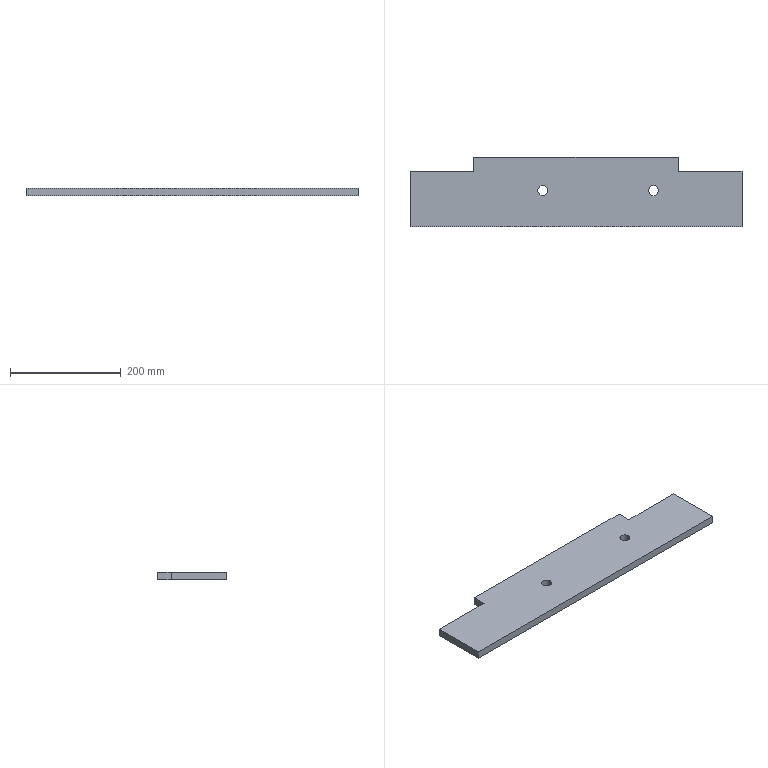Part | SolidWorks | features Extrusion 1 | 1 solid | 14 faces | box 600 x 125 x 14 mm | volume 962375 mm3 | plane 10 | cylinder 4 | commonest cylinder face diameters 18 x4
STEP:
#1=CARTESIAN_POINT('',(431.,65.,14.));
#2=VERTEX_POINT('',#1);
#3=CARTESIAN_POINT('',(449.,65.,14.));
#4=VERTEX_POINT('',#3);
#5=CARTESIAN_POINT('',(440.,65.,14.));
#6=DIRECTION('',(0.,0.,1.));
#7=DIRECTION('',(1.,0.,0.));
#8=AXIS2_PLACEMENT_3D('',#5,#6,#7);
#9=CIRCLE('',#8,9.);
#10=EDGE_CURVE('',#2,#4,#9,.T.);
#11=ORIENTED_EDGE('',*,*,#10,.T.);
#12=CARTESIAN_POINT('',(449.,65.,0.));
#13=VERTEX_POINT('',#12);
#14=CARTESIAN_POINT('',(449.,65.,14.));
#15=DIRECTION('',(0.,0.,-1.));
#16=VECTOR('',#15,1000.);
#17=LINE('',#14,#16);
#18=EDGE_CURVE('',#4,#13,#17,.T.);
#19=ORIENTED_EDGE('',*,*,#18,.T.);
#20=CARTESIAN_POINT('',(431.,65.,0.));
#21=VERTEX_POINT('',#20);
#22=CARTESIAN_POINT('',(440.,65.,0.));
#23=DIRECTION('',(0.,0.,1.));
#24=DIRECTION('',(1.,0.,0.));
#25=AXIS2_PLACEMENT_3D('',#22,#23,#24);
#26=CIRCLE('',#25,9.);
#27=EDGE_CURVE('',#21,#13,#26,.T.);
#28=ORIENTED_EDGE('',*,*,#27,.F.);
#29=CARTESIAN_POINT('',(431.,65.,14.));
#30=DIRECTION('',(0.,0.,-1.));
#31=VECTOR('',#30,1000.);
#32=LINE('',#29,#31);
#33=EDGE_CURVE('',#2,#21,#32,.T.);
#34=ORIENTED_EDGE('',*,*,#33,.F.);
#35=EDGE_LOOP('',(#11,#19,#28,#34));
#36=FACE_OUTER_BOUND('',#35,.T.);
#37=CARTESIAN_POINT('',(440.,65.,14.));
#38=DIRECTION('',(0.,0.,-1.));
#39=DIRECTION('',(-1.,0.,0.));
#40=AXIS2_PLACEMENT_3D('',#37,#38,#39);
#41=CYLINDRICAL_SURFACE('',#40,9.);
#42=ADVANCED_FACE('',(#36),#41,.F.);
#43=CARTESIAN_POINT('',(231.,65.,14.));
#44=VERTEX_POINT('',#43);
#45=CARTESIAN_POINT('',(249.,65.,14.));
#46=VERTEX_POINT('',#45);
#47=CARTESIAN_POINT('',(240.,65.,14.));
#48=DIRECTION('',(0.,0.,1.));
#49=DIRECTION('',(1.,0.,0.));
#50=AXIS2_PLACEMENT_3D('',#47,#48,#49);
#51=CIRCLE('',#50,9.);
#52=EDGE_CURVE('',#44,#46,#51,.T.);
#53=ORIENTED_EDGE('',*,*,#52,.T.);
#54=CARTESIAN_POINT('',(249.,65.,0.));
#55=VERTEX_POINT('',#54);
#56=CARTESIAN_POINT('',(249.,65.,14.));
#57=DIRECTION('',(0.,0.,-1.));
#58=VECTOR('',#57,1000.);
#59=LINE('',#56,#58);
#60=EDGE_CURVE('',#46,#55,#59,.T.);
#61=ORIENTED_EDGE('',*,*,#60,.T.);
#62=CARTESIAN_POINT('',(231.,65.,0.));
#63=VERTEX_POINT('',#62);
#64=CARTESIAN_POINT('',(240.,65.,0.));
#65=DIRECTION('',(0.,0.,1.));
#66=DIRECTION('',(1.,0.,0.));
#67=AXIS2_PLACEMENT_3D('',#64,#65,#66);
#68=CIRCLE('',#67,9.);
#69=EDGE_CURVE('',#63,#55,#68,.T.);
#70=ORIENTED_EDGE('',*,*,#69,.F.);
#71=CARTESIAN_POINT('',(231.,65.,14.));
#72=DIRECTION('',(0.,0.,-1.));
#73=VECTOR('',#72,1000.);
#74=LINE('',#71,#73);
#75=EDGE_CURVE('',#44,#63,#74,.T.);
#76=ORIENTED_EDGE('',*,*,#75,.F.);
#77=EDGE_LOOP('',(#53,#61,#70,#76));
#78=FACE_OUTER_BOUND('',#77,.T.);
#79=CARTESIAN_POINT('',(240.,65.,14.));
#80=DIRECTION('',(0.,0.,-1.));
#81=DIRECTION('',(-1.,0.,0.));
#82=AXIS2_PLACEMENT_3D('',#79,#80,#81);
#83=CYLINDRICAL_SURFACE('',#82,9.);
#84=ADVANCED_FACE('',(#78),#83,.F.);
#85=CARTESIAN_POINT('',(0.,0.,14.));
#86=VERTEX_POINT('',#85);
#87=CARTESIAN_POINT('',(600.,0.,14.));
#88=VERTEX_POINT('',#87);
#89=CARTESIAN_POINT('',(600.,0.,14.));
#90=DIRECTION('',(1.,0.,0.));
#91=VECTOR('',#90,1000.);
#92=LINE('',#89,#91);
#93=EDGE_CURVE('',#86,#88,#92,.T.);
#94=ORIENTED_EDGE('',*,*,#93,.T.);
#95=CARTESIAN_POINT('',(600.,100.,14.));
#96=VERTEX_POINT('',#95);
#97=CARTESIAN_POINT('',(600.,100.,14.));
#98=DIRECTION('',(0.,1.,0.));
#99=VECTOR('',#98,1000.);
#100=LINE('',#97,#99);
#101=EDGE_CURVE('',#88,#96,#100,.T.);
#102=ORIENTED_EDGE('',*,*,#101,.T.);
#103=CARTESIAN_POINT('',(485.,100.,14.));
#104=VERTEX_POINT('',#103);
#105=CARTESIAN_POINT('',(485.,100.,14.));
#106=DIRECTION('',(-1.,0.,0.));
#107=VECTOR('',#106,1000.);
#108=LINE('',#105,#107);
#109=EDGE_CURVE('',#96,#104,#108,.T.);
#110=ORIENTED_EDGE('',*,*,#109,.T.);
#111=CARTESIAN_POINT('',(485.,125.,14.));
#112=VERTEX_POINT('',#111);
#113=CARTESIAN_POINT('',(485.,125.,14.));
#114=DIRECTION('',(0.,1.,0.));
#115=VECTOR('',#114,1000.);
#116=LINE('',#113,#115);
#117=EDGE_CURVE('',#104,#112,#116,.T.);
#118=ORIENTED_EDGE('',*,*,#117,.T.);
#119=CARTESIAN_POINT('',(115.,125.,14.));
#120=VERTEX_POINT('',#119);
#121=CARTESIAN_POINT('',(115.,125.,14.));
#122=DIRECTION('',(-1.,0.,0.));
#123=VECTOR('',#122,1000.);
#124=LINE('',#121,#123);
#125=EDGE_CURVE('',#112,#120,#124,.T.);
#126=ORIENTED_EDGE('',*,*,#125,.T.);
#127=CARTESIAN_POINT('',(115.,100.,14.));
#128=VERTEX_POINT('',#127);
#129=CARTESIAN_POINT('',(115.,100.,14.));
#130=DIRECTION('',(0.,-1.,0.));
#131=VECTOR('',#130,1000.);
#132=LINE('',#129,#131);
#133=EDGE_CURVE('',#120,#128,#132,.T.);
#134=ORIENTED_EDGE('',*,*,#133,.T.);
#135=CARTESIAN_POINT('',(0.,100.,14.));
#136=VERTEX_POINT('',#135);
#137=CARTESIAN_POINT('',(0.,100.,14.));
#138=DIRECTION('',(-1.,0.,0.));
#139=VECTOR('',#138,1000.);
#140=LINE('',#137,#139);
#141=EDGE_CURVE('',#128,#136,#140,.T.);
#142=ORIENTED_EDGE('',*,*,#141,.T.);
#143=CARTESIAN_POINT('',(0.,0.,14.));
#144=DIRECTION('',(0.,-1.,0.));
#145=VECTOR('',#144,1000.);
#146=LINE('',#143,#145);
#147=EDGE_CURVE('',#136,#86,#146,.T.);
#148=ORIENTED_EDGE('',*,*,#147,.T.);
#149=EDGE_LOOP('',(#94,#102,#110,#118,#126,#134,#142,#148));
#150=FACE_OUTER_BOUND('',#149,.T.);
#151=ORIENTED_EDGE('',*,*,#52,.F.);
#152=CARTESIAN_POINT('',(240.,65.,14.));
#153=DIRECTION('',(0.,0.,1.));
#154=DIRECTION('',(1.,0.,0.));
#155=AXIS2_PLACEMENT_3D('',#152,#153,#154);
#156=CIRCLE('',#155,9.);
#157=EDGE_CURVE('',#46,#44,#156,.T.);
#158=ORIENTED_EDGE('',*,*,#157,.F.);
#159=EDGE_LOOP('',(#151,#158));
#160=FACE_BOUND('',#159,.T.);
#161=ORIENTED_EDGE('',*,*,#10,.F.);
#162=CARTESIAN_POINT('',(440.,65.,14.));
#163=DIRECTION('',(0.,0.,1.));
#164=DIRECTION('',(1.,0.,0.));
#165=AXIS2_PLACEMENT_3D('',#162,#163,#164);
#166=CIRCLE('',#165,9.);
#167=EDGE_CURVE('',#4,#2,#166,.T.);
#168=ORIENTED_EDGE('',*,*,#167,.F.);
#169=EDGE_LOOP('',(#161,#168));
#170=FACE_BOUND('',#169,.T.);
#171=CARTESIAN_POINT('',(0.,0.,14.));
#172=DIRECTION('',(0.,0.,-1.));
#173=DIRECTION('',(-1.,0.,0.));
#174=AXIS2_PLACEMENT_3D('',#171,#172,#173);
#175=PLANE('',#174);
#176=ADVANCED_FACE('',(#150,#160,#170),#175,.F.);
#177=ORIENTED_EDGE('',*,*,#69,.T.);
#178=CARTESIAN_POINT('',(240.,65.,0.));
#179=DIRECTION('',(0.,0.,1.));
#180=DIRECTION('',(1.,0.,0.));
#181=AXIS2_PLACEMENT_3D('',#178,#179,#180);
#182=CIRCLE('',#181,9.);
#183=EDGE_CURVE('',#55,#63,#182,.T.);
#184=ORIENTED_EDGE('',*,*,#183,.T.);
#185=EDGE_LOOP('',(#177,#184));
#186=FACE_BOUND('',#185,.T.);
#187=CARTESIAN_POINT('',(0.,0.,0.));
#188=VERTEX_POINT('',#187);
#189=CARTESIAN_POINT('',(600.,0.,0.));
#190=VERTEX_POINT('',#189);
#191=CARTESIAN_POINT('',(600.,0.,0.));
#192=DIRECTION('',(1.,0.,0.));
#193=VECTOR('',#192,1000.);
#194=LINE('',#191,#193);
#195=EDGE_CURVE('',#188,#190,#194,.T.);
#196=ORIENTED_EDGE('',*,*,#195,.F.);
#197=CARTESIAN_POINT('',(0.,100.,0.));
#198=VERTEX_POINT('',#197);
#199=CARTESIAN_POINT('',(0.,0.,0.));
#200=DIRECTION('',(0.,-1.,0.));
#201=VECTOR('',#200,1000.);
#202=LINE('',#199,#201);
#203=EDGE_CURVE('',#198,#188,#202,.T.);
#204=ORIENTED_EDGE('',*,*,#203,.F.);
#205=CARTESIAN_POINT('',(115.,100.,0.));
#206=VERTEX_POINT('',#205);
#207=CARTESIAN_POINT('',(0.,100.,0.));
#208=DIRECTION('',(-1.,0.,0.));
#209=VECTOR('',#208,1000.);
#210=LINE('',#207,#209);
#211=EDGE_CURVE('',#206,#198,#210,.T.);
#212=ORIENTED_EDGE('',*,*,#211,.F.);
#213=CARTESIAN_POINT('',(115.,125.,0.));
#214=VERTEX_POINT('',#213);
#215=CARTESIAN_POINT('',(115.,100.,0.));
#216=DIRECTION('',(0.,-1.,0.));
#217=VECTOR('',#216,1000.);
#218=LINE('',#215,#217);
#219=EDGE_CURVE('',#214,#206,#218,.T.);
#220=ORIENTED_EDGE('',*,*,#219,.F.);
#221=CARTESIAN_POINT('',(485.,125.,0.));
#222=VERTEX_POINT('',#221);
#223=CARTESIAN_POINT('',(115.,125.,0.));
#224=DIRECTION('',(-1.,0.,0.));
#225=VECTOR('',#224,1000.);
#226=LINE('',#223,#225);
#227=EDGE_CURVE('',#222,#214,#226,.T.);
#228=ORIENTED_EDGE('',*,*,#227,.F.);
#229=CARTESIAN_POINT('',(485.,100.,0.));
#230=VERTEX_POINT('',#229);
#231=CARTESIAN_POINT('',(485.,125.,0.));
#232=DIRECTION('',(0.,1.,0.));
#233=VECTOR('',#232,1000.);
#234=LINE('',#231,#233);
#235=EDGE_CURVE('',#230,#222,#234,.T.);
#236=ORIENTED_EDGE('',*,*,#235,.F.);
#237=CARTESIAN_POINT('',(600.,100.,0.));
#238=VERTEX_POINT('',#237);
#239=CARTESIAN_POINT('',(485.,100.,0.));
#240=DIRECTION('',(-1.,0.,0.));
#241=VECTOR('',#240,1000.);
#242=LINE('',#239,#241);
#243=EDGE_CURVE('',#238,#230,#242,.T.);
#244=ORIENTED_EDGE('',*,*,#243,.F.);
#245=CARTESIAN_POINT('',(600.,100.,0.));
#246=DIRECTION('',(0.,1.,0.));
#247=VECTOR('',#246,1000.);
#248=LINE('',#245,#247);
#249=EDGE_CURVE('',#190,#238,#248,.T.);
#250=ORIENTED_EDGE('',*,*,#249,.F.);
#251=EDGE_LOOP('',(#196,#204,#212,#220,#228,#236,#244,#250));
#252=FACE_OUTER_BOUND('',#251,.T.);
#253=ORIENTED_EDGE('',*,*,#27,.T.);
#254=CARTESIAN_POINT('',(440.,65.,0.));
#255=DIRECTION('',(0.,0.,1.));
#256=DIRECTION('',(1.,0.,0.));
#257=AXIS2_PLACEMENT_3D('',#254,#255,#256);
#258=CIRCLE('',#257,9.);
#259=EDGE_CURVE('',#13,#21,#258,.T.);
#260=ORIENTED_EDGE('',*,*,#259,.T.);
#261=EDGE_LOOP('',(#253,#260));
#262=FACE_BOUND('',#261,.T.);
#263=CARTESIAN_POINT('',(0.,0.,0.));
#264=DIRECTION('',(0.,0.,-1.));
#265=DIRECTION('',(-1.,0.,0.));
#266=AXIS2_PLACEMENT_3D('',#263,#264,#265);
#267=PLANE('',#266);
#268=ADVANCED_FACE('',(#186,#252,#262),#267,.T.);
#269=ORIENTED_EDGE('',*,*,#195,.T.);
#270=CARTESIAN_POINT('',(600.,0.,14.));
#271=DIRECTION('',(0.,0.,-1.));
#272=VECTOR('',#271,1000.);
#273=LINE('',#270,#272);
#274=EDGE_CURVE('',#88,#190,#273,.T.);
#275=ORIENTED_EDGE('',*,*,#274,.F.);
#276=ORIENTED_EDGE('',*,*,#93,.F.);
#277=CARTESIAN_POINT('',(0.,0.,14.));
#278=DIRECTION('',(0.,0.,-1.));
#279=VECTOR('',#278,1000.);
#280=LINE('',#277,#279);
#281=EDGE_CURVE('',#86,#188,#280,.T.);
#282=ORIENTED_EDGE('',*,*,#281,.T.);
#283=EDGE_LOOP('',(#269,#275,#276,#282));
#284=FACE_OUTER_BOUND('',#283,.T.);
#285=CARTESIAN_POINT('',(600.,0.,14.));
#286=DIRECTION('',(0.,1.,0.));
#287=DIRECTION('',(0.,0.,1.));
#288=AXIS2_PLACEMENT_3D('',#285,#286,#287);
#289=PLANE('',#288);
#290=ADVANCED_FACE('',(#284),#289,.F.);
#291=ORIENTED_EDGE('',*,*,#249,.T.);
#292=CARTESIAN_POINT('',(600.,100.,14.));
#293=DIRECTION('',(0.,0.,-1.));
#294=VECTOR('',#293,1000.);
#295=LINE('',#292,#294);
#296=EDGE_CURVE('',#96,#238,#295,.T.);
#297=ORIENTED_EDGE('',*,*,#296,.F.);
#298=ORIENTED_EDGE('',*,*,#101,.F.);
#299=ORIENTED_EDGE('',*,*,#274,.T.);
#300=EDGE_LOOP('',(#291,#297,#298,#299));
#301=FACE_OUTER_BOUND('',#300,.T.);
#302=CARTESIAN_POINT('',(600.,100.,14.));
#303=DIRECTION('',(-1.,0.,0.));
#304=DIRECTION('',(0.,0.,1.));
#305=AXIS2_PLACEMENT_3D('',#302,#303,#304);
#306=PLANE('',#305);
#307=ADVANCED_FACE('',(#301),#306,.F.);
#308=ORIENTED_EDGE('',*,*,#243,.T.);
#309=CARTESIAN_POINT('',(485.,100.,14.));
#310=DIRECTION('',(0.,0.,-1.));
#311=VECTOR('',#310,1000.);
#312=LINE('',#309,#311);
#313=EDGE_CURVE('',#104,#230,#312,.T.);
#314=ORIENTED_EDGE('',*,*,#313,.F.);
#315=ORIENTED_EDGE('',*,*,#109,.F.);
#316=ORIENTED_EDGE('',*,*,#296,.T.);
#317=EDGE_LOOP('',(#308,#314,#315,#316));
#318=FACE_OUTER_BOUND('',#317,.T.);
#319=CARTESIAN_POINT('',(485.,100.,14.));
#320=DIRECTION('',(0.,-1.,0.));
#321=DIRECTION('',(0.,0.,-1.));
#322=AXIS2_PLACEMENT_3D('',#319,#320,#321);
#323=PLANE('',#322);
#324=ADVANCED_FACE('',(#318),#323,.F.);
#325=ORIENTED_EDGE('',*,*,#235,.T.);
#326=CARTESIAN_POINT('',(485.,125.,14.));
#327=DIRECTION('',(0.,0.,-1.));
#328=VECTOR('',#327,1000.);
#329=LINE('',#326,#328);
#330=EDGE_CURVE('',#112,#222,#329,.T.);
#331=ORIENTED_EDGE('',*,*,#330,.F.);
#332=ORIENTED_EDGE('',*,*,#117,.F.);
#333=ORIENTED_EDGE('',*,*,#313,.T.);
#334=EDGE_LOOP('',(#325,#331,#332,#333));
#335=FACE_OUTER_BOUND('',#334,.T.);
#336=CARTESIAN_POINT('',(485.,125.,14.));
#337=DIRECTION('',(-1.,0.,0.));
#338=DIRECTION('',(0.,0.,1.));
#339=AXIS2_PLACEMENT_3D('',#336,#337,#338);
#340=PLANE('',#339);
#341=ADVANCED_FACE('',(#335),#340,.F.);
#342=ORIENTED_EDGE('',*,*,#227,.T.);
#343=CARTESIAN_POINT('',(115.,125.,14.));
#344=DIRECTION('',(0.,0.,-1.));
#345=VECTOR('',#344,1000.);
#346=LINE('',#343,#345);
#347=EDGE_CURVE('',#120,#214,#346,.T.);
#348=ORIENTED_EDGE('',*,*,#347,.F.);
#349=ORIENTED_EDGE('',*,*,#125,.F.);
#350=ORIENTED_EDGE('',*,*,#330,.T.);
#351=EDGE_LOOP('',(#342,#348,#349,#350));
#352=FACE_OUTER_BOUND('',#351,.T.);
#353=CARTESIAN_POINT('',(115.,125.,14.));
#354=DIRECTION('',(0.,-1.,0.));
#355=DIRECTION('',(0.,0.,-1.));
#356=AXIS2_PLACEMENT_3D('',#353,#354,#355);
#357=PLANE('',#356);
#358=ADVANCED_FACE('',(#352),#357,.F.);
#359=ORIENTED_EDGE('',*,*,#219,.T.);
#360=CARTESIAN_POINT('',(115.,100.,14.));
#361=DIRECTION('',(0.,0.,-1.));
#362=VECTOR('',#361,1000.);
#363=LINE('',#360,#362);
#364=EDGE_CURVE('',#128,#206,#363,.T.);
#365=ORIENTED_EDGE('',*,*,#364,.F.);
#366=ORIENTED_EDGE('',*,*,#133,.F.);
#367=ORIENTED_EDGE('',*,*,#347,.T.);
#368=EDGE_LOOP('',(#359,#365,#366,#367));
#369=FACE_OUTER_BOUND('',#368,.T.);
#370=CARTESIAN_POINT('',(115.,100.,14.));
#371=DIRECTION('',(1.,0.,0.));
#372=DIRECTION('',(0.,0.,-1.));
#373=AXIS2_PLACEMENT_3D('',#370,#371,#372);
#374=PLANE('',#373);
#375=ADVANCED_FACE('',(#369),#374,.F.);
#376=ORIENTED_EDGE('',*,*,#211,.T.);
#377=CARTESIAN_POINT('',(0.,100.,14.));
#378=DIRECTION('',(0.,0.,-1.));
#379=VECTOR('',#378,1000.);
#380=LINE('',#377,#379);
#381=EDGE_CURVE('',#136,#198,#380,.T.);
#382=ORIENTED_EDGE('',*,*,#381,.F.);
#383=ORIENTED_EDGE('',*,*,#141,.F.);
#384=ORIENTED_EDGE('',*,*,#364,.T.);
#385=EDGE_LOOP('',(#376,#382,#383,#384));
#386=FACE_OUTER_BOUND('',#385,.T.);
#387=CARTESIAN_POINT('',(0.,100.,14.));
#388=DIRECTION('',(0.,-1.,0.));
#389=DIRECTION('',(0.,0.,-1.));
#390=AXIS2_PLACEMENT_3D('',#387,#388,#389);
#391=PLANE('',#390);
#392=ADVANCED_FACE('',(#386),#391,.F.);
#393=ORIENTED_EDGE('',*,*,#203,.T.);
#394=ORIENTED_EDGE('',*,*,#281,.F.);
#395=ORIENTED_EDGE('',*,*,#147,.F.);
#396=ORIENTED_EDGE('',*,*,#381,.T.);
#397=EDGE_LOOP('',(#393,#394,#395,#396));
#398=FACE_OUTER_BOUND('',#397,.T.);
#399=CARTESIAN_POINT('',(0.,0.,14.));
#400=DIRECTION('',(1.,0.,0.));
#401=DIRECTION('',(0.,0.,-1.));
#402=AXIS2_PLACEMENT_3D('',#399,#400,#401);
#403=PLANE('',#402);
#404=ADVANCED_FACE('',(#398),#403,.F.);
#405=ORIENTED_EDGE('',*,*,#60,.F.);
#406=ORIENTED_EDGE('',*,*,#157,.T.);
#407=ORIENTED_EDGE('',*,*,#75,.T.);
#408=ORIENTED_EDGE('',*,*,#183,.F.);
#409=EDGE_LOOP('',(#405,#406,#407,#408));
#410=FACE_OUTER_BOUND('',#409,.T.);
#411=CARTESIAN_POINT('',(240.,65.,14.));
#412=DIRECTION('',(0.,0.,-1.));
#413=DIRECTION('',(-1.,0.,0.));
#414=AXIS2_PLACEMENT_3D('',#411,#412,#413);
#415=CYLINDRICAL_SURFACE('',#414,9.);
#416=ADVANCED_FACE('',(#410),#415,.F.);
#417=ORIENTED_EDGE('',*,*,#18,.F.);
#418=ORIENTED_EDGE('',*,*,#167,.T.);
#419=ORIENTED_EDGE('',*,*,#33,.T.);
#420=ORIENTED_EDGE('',*,*,#259,.F.);
#421=EDGE_LOOP('',(#417,#418,#419,#420));
#422=FACE_OUTER_BOUND('',#421,.T.);
#423=CARTESIAN_POINT('',(440.,65.,14.));
#424=DIRECTION('',(0.,0.,-1.));
#425=DIRECTION('',(-1.,0.,0.));
#426=AXIS2_PLACEMENT_3D('',#423,#424,#425);
#427=CYLINDRICAL_SURFACE('',#426,9.);
#428=ADVANCED_FACE('',(#422),#427,.F.);
#429=CLOSED_SHELL('',(#42,#84,#176,#268,#290,#307,#324,#341,#358,#375,#392,#404,#416,#428));
#430=MANIFOLD_SOLID_BREP('',#429);
#431=CARTESIAN_POINT('',(0.,0.,0.));
#432=DIRECTION('',(0.,0.,1.));
#433=DIRECTION('',(1.,0.,0.));
#434=AXIS2_PLACEMENT_3D('',#431,#432,#433);
#435=(LENGTH_UNIT()NAMED_UNIT(*)SI_UNIT(.MILLI.,.METRE.));
#436=UNCERTAINTY_MEASURE_WITH_UNIT(LENGTH_MEASURE(0.00001),#435,'','');
#437=(NAMED_UNIT(*)PLANE_ANGLE_UNIT()SI_UNIT($,.RADIAN.));
#438=(NAMED_UNIT(*)SI_UNIT($,.STERADIAN.)SOLID_ANGLE_UNIT());
#439=(GEOMETRIC_REPRESENTATION_CONTEXT(3)GLOBAL_UNCERTAINTY_ASSIGNED_CONTEXT((#436))GLOBAL_UNIT_ASSIGNED_CONTEXT((#435,#437,#438))REPRESENTATION_CONTEXT('',''));
#440=ADVANCED_BREP_SHAPE_REPRESENTATION('',(#430,#434),#439);